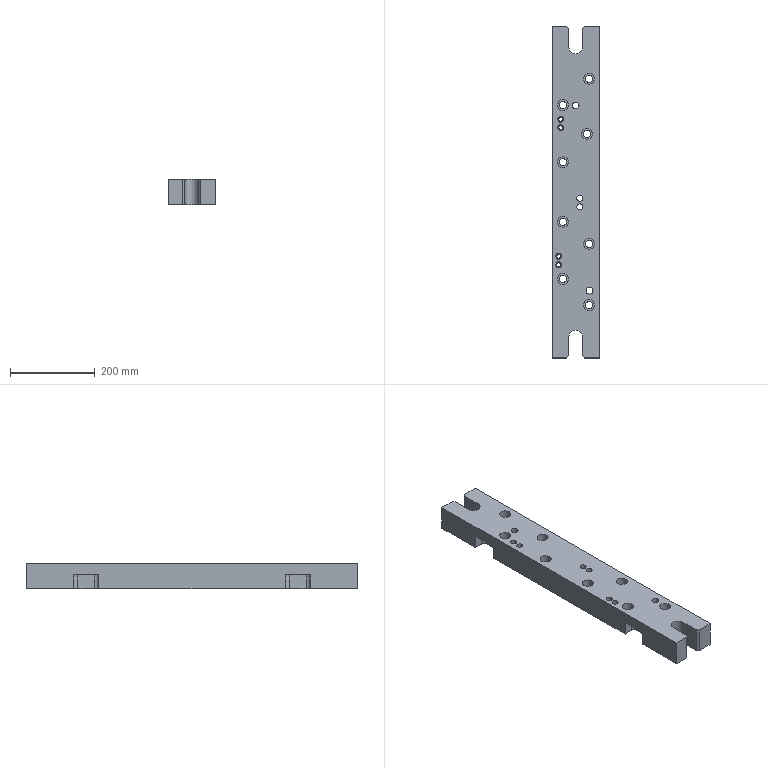Part | STEP file | PN_0006_id1766_x_t | 1 solid | 74 faces | box 112 x 785 x 60 mm | volume 4657225 mm3 | plane 38 | cylinder 36 | commonest cylinder face diameters 17 x8 26 x8 14 x6 9 x4 20 x4 16 x2